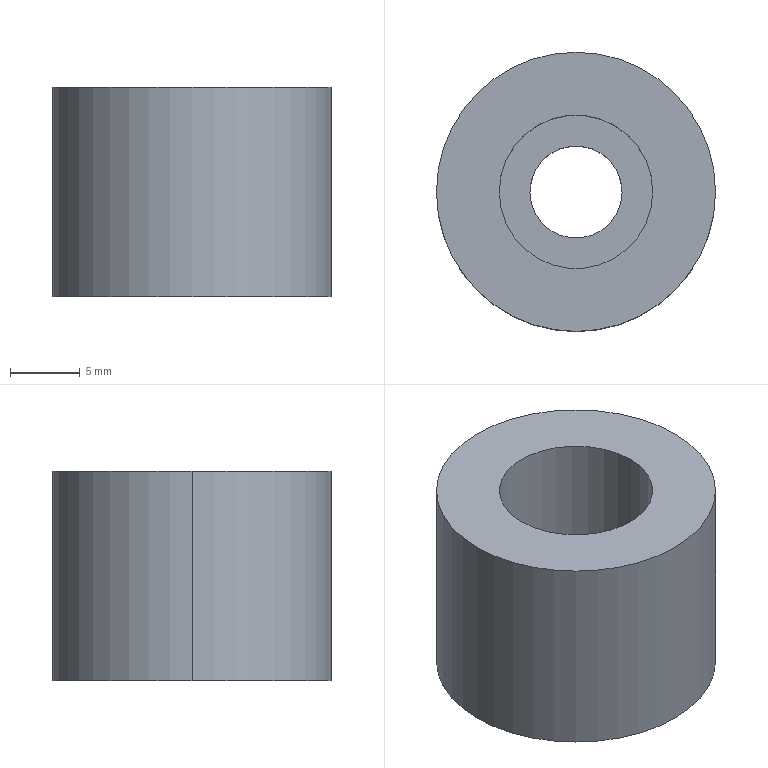Part | SolidWorks | features Extrusion 1, HoleWzd 1 | 1 solid | 9 faces | box 20 x 20 x 15 mm | volume 3713 mm3 | cylinder 6 | plane 3 | commonest cylinder face diameters 6.6 x2 11 x2 20 x2
STEP:
#1=CARTESIAN_POINT('',(-5.5,0.,7.));
#2=VERTEX_POINT('',#1);
#3=CARTESIAN_POINT('',(5.5,0.,7.));
#4=VERTEX_POINT('',#3);
#5=CARTESIAN_POINT('',(0.,0.,7.));
#6=DIRECTION('',(0.,0.,1.));
#7=DIRECTION('',(1.,0.,0.));
#8=AXIS2_PLACEMENT_3D('',#5,#6,#7);
#9=CIRCLE('',#8,5.5);
#10=EDGE_CURVE('',#2,#4,#9,.T.);
#11=ORIENTED_EDGE('',*,*,#10,.F.);
#12=CARTESIAN_POINT('',(-5.5,0.,15.));
#13=VERTEX_POINT('',#12);
#14=CARTESIAN_POINT('',(-5.5,0.,15.));
#15=DIRECTION('',(0.,0.,1.));
#16=VECTOR('',#15,1000.);
#17=LINE('',#14,#16);
#18=EDGE_CURVE('',#2,#13,#17,.T.);
#19=ORIENTED_EDGE('',*,*,#18,.T.);
#20=CARTESIAN_POINT('',(5.5,0.,15.));
#21=VERTEX_POINT('',#20);
#22=CARTESIAN_POINT('',(0.,0.,15.));
#23=DIRECTION('',(0.,0.,1.));
#24=DIRECTION('',(1.,0.,0.));
#25=AXIS2_PLACEMENT_3D('',#22,#23,#24);
#26=CIRCLE('',#25,5.5);
#27=EDGE_CURVE('',#13,#21,#26,.T.);
#28=ORIENTED_EDGE('',*,*,#27,.T.);
#29=CARTESIAN_POINT('',(5.5,0.,15.));
#30=DIRECTION('',(0.,0.,1.));
#31=VECTOR('',#30,1000.);
#32=LINE('',#29,#31);
#33=EDGE_CURVE('',#4,#21,#32,.T.);
#34=ORIENTED_EDGE('',*,*,#33,.F.);
#35=EDGE_LOOP('',(#11,#19,#28,#34));
#36=FACE_OUTER_BOUND('',#35,.T.);
#37=CARTESIAN_POINT('',(0.,0.,15.));
#38=DIRECTION('',(0.,0.,1.));
#39=DIRECTION('',(1.,0.,0.));
#40=AXIS2_PLACEMENT_3D('',#37,#38,#39);
#41=CYLINDRICAL_SURFACE('',#40,5.5);
#42=ADVANCED_FACE('',(#36),#41,.F.);
#43=CARTESIAN_POINT('',(-3.3,0.,0.));
#44=VERTEX_POINT('',#43);
#45=CARTESIAN_POINT('',(3.3,0.,0.));
#46=VERTEX_POINT('',#45);
#47=CARTESIAN_POINT('',(0.,0.,0.));
#48=DIRECTION('',(0.,0.,1.));
#49=DIRECTION('',(1.,0.,0.));
#50=AXIS2_PLACEMENT_3D('',#47,#48,#49);
#51=CIRCLE('',#50,3.3);
#52=EDGE_CURVE('',#44,#46,#51,.T.);
#53=ORIENTED_EDGE('',*,*,#52,.F.);
#54=CARTESIAN_POINT('',(-3.3,0.,7.));
#55=VERTEX_POINT('',#54);
#56=CARTESIAN_POINT('',(-3.3,0.,15.));
#57=DIRECTION('',(0.,0.,1.));
#58=VECTOR('',#57,1000.);
#59=LINE('',#56,#58);
#60=EDGE_CURVE('',#44,#55,#59,.T.);
#61=ORIENTED_EDGE('',*,*,#60,.T.);
#62=CARTESIAN_POINT('',(3.3,0.,7.));
#63=VERTEX_POINT('',#62);
#64=CARTESIAN_POINT('',(0.,0.,7.));
#65=DIRECTION('',(0.,0.,1.));
#66=DIRECTION('',(1.,0.,0.));
#67=AXIS2_PLACEMENT_3D('',#64,#65,#66);
#68=CIRCLE('',#67,3.3);
#69=EDGE_CURVE('',#55,#63,#68,.T.);
#70=ORIENTED_EDGE('',*,*,#69,.T.);
#71=CARTESIAN_POINT('',(3.3,0.,15.));
#72=DIRECTION('',(0.,0.,1.));
#73=VECTOR('',#72,1000.);
#74=LINE('',#71,#73);
#75=EDGE_CURVE('',#46,#63,#74,.T.);
#76=ORIENTED_EDGE('',*,*,#75,.F.);
#77=EDGE_LOOP('',(#53,#61,#70,#76));
#78=FACE_OUTER_BOUND('',#77,.T.);
#79=CARTESIAN_POINT('',(0.,0.,15.));
#80=DIRECTION('',(0.,0.,1.));
#81=DIRECTION('',(1.,0.,0.));
#82=AXIS2_PLACEMENT_3D('',#79,#80,#81);
#83=CYLINDRICAL_SURFACE('',#82,3.3);
#84=ADVANCED_FACE('',(#78),#83,.F.);
#85=CARTESIAN_POINT('',(10.,0.,15.));
#86=VERTEX_POINT('',#85);
#87=CARTESIAN_POINT('',(-10.,0.,15.));
#88=VERTEX_POINT('',#87);
#89=CARTESIAN_POINT('',(0.,0.,15.));
#90=DIRECTION('',(0.,0.,1.));
#91=DIRECTION('',(1.,0.,0.));
#92=AXIS2_PLACEMENT_3D('',#89,#90,#91);
#93=CIRCLE('',#92,10.);
#94=EDGE_CURVE('',#86,#88,#93,.T.);
#95=ORIENTED_EDGE('',*,*,#94,.F.);
#96=CARTESIAN_POINT('',(10.,0.,0.));
#97=VERTEX_POINT('',#96);
#98=CARTESIAN_POINT('',(10.,0.,15.));
#99=DIRECTION('',(0.,0.,-1.));
#100=VECTOR('',#99,1000.);
#101=LINE('',#98,#100);
#102=EDGE_CURVE('',#86,#97,#101,.T.);
#103=ORIENTED_EDGE('',*,*,#102,.T.);
#104=CARTESIAN_POINT('',(-10.,0.,0.));
#105=VERTEX_POINT('',#104);
#106=CARTESIAN_POINT('',(0.,0.,0.));
#107=DIRECTION('',(0.,0.,1.));
#108=DIRECTION('',(1.,0.,0.));
#109=AXIS2_PLACEMENT_3D('',#106,#107,#108);
#110=CIRCLE('',#109,10.);
#111=EDGE_CURVE('',#97,#105,#110,.T.);
#112=ORIENTED_EDGE('',*,*,#111,.T.);
#113=CARTESIAN_POINT('',(-10.,0.,15.));
#114=DIRECTION('',(0.,0.,-1.));
#115=VECTOR('',#114,1000.);
#116=LINE('',#113,#115);
#117=EDGE_CURVE('',#88,#105,#116,.T.);
#118=ORIENTED_EDGE('',*,*,#117,.F.);
#119=EDGE_LOOP('',(#95,#103,#112,#118));
#120=FACE_OUTER_BOUND('',#119,.T.);
#121=CARTESIAN_POINT('',(0.,0.,15.));
#122=DIRECTION('',(0.,0.,-1.));
#123=DIRECTION('',(-1.,0.,0.));
#124=AXIS2_PLACEMENT_3D('',#121,#122,#123);
#125=CYLINDRICAL_SURFACE('',#124,10.);
#126=ADVANCED_FACE('',(#120),#125,.T.);
#127=ORIENTED_EDGE('',*,*,#102,.F.);
#128=CARTESIAN_POINT('',(0.,0.,15.));
#129=DIRECTION('',(0.,0.,1.));
#130=DIRECTION('',(1.,0.,0.));
#131=AXIS2_PLACEMENT_3D('',#128,#129,#130);
#132=CIRCLE('',#131,10.);
#133=EDGE_CURVE('',#88,#86,#132,.T.);
#134=ORIENTED_EDGE('',*,*,#133,.F.);
#135=ORIENTED_EDGE('',*,*,#117,.T.);
#136=CARTESIAN_POINT('',(0.,0.,0.));
#137=DIRECTION('',(0.,0.,1.));
#138=DIRECTION('',(1.,0.,0.));
#139=AXIS2_PLACEMENT_3D('',#136,#137,#138);
#140=CIRCLE('',#139,10.);
#141=EDGE_CURVE('',#105,#97,#140,.T.);
#142=ORIENTED_EDGE('',*,*,#141,.T.);
#143=EDGE_LOOP('',(#127,#134,#135,#142));
#144=FACE_OUTER_BOUND('',#143,.T.);
#145=CARTESIAN_POINT('',(0.,0.,15.));
#146=DIRECTION('',(0.,0.,-1.));
#147=DIRECTION('',(-1.,0.,0.));
#148=AXIS2_PLACEMENT_3D('',#145,#146,#147);
#149=CYLINDRICAL_SURFACE('',#148,10.);
#150=ADVANCED_FACE('',(#144),#149,.T.);
#151=CARTESIAN_POINT('',(0.,0.,15.));
#152=DIRECTION('',(0.,0.,1.));
#153=DIRECTION('',(1.,0.,0.));
#154=AXIS2_PLACEMENT_3D('',#151,#152,#153);
#155=CIRCLE('',#154,5.5);
#156=EDGE_CURVE('',#21,#13,#155,.T.);
#157=ORIENTED_EDGE('',*,*,#156,.F.);
#158=ORIENTED_EDGE('',*,*,#27,.F.);
#159=EDGE_LOOP('',(#157,#158));
#160=FACE_BOUND('',#159,.T.);
#161=ORIENTED_EDGE('',*,*,#133,.T.);
#162=ORIENTED_EDGE('',*,*,#94,.T.);
#163=EDGE_LOOP('',(#161,#162));
#164=FACE_OUTER_BOUND('',#163,.T.);
#165=CARTESIAN_POINT('',(0.,0.,15.));
#166=DIRECTION('',(0.,0.,1.));
#167=DIRECTION('',(1.,0.,0.));
#168=AXIS2_PLACEMENT_3D('',#165,#166,#167);
#169=PLANE('',#168);
#170=ADVANCED_FACE('',(#160,#164),#169,.T.);
#171=CARTESIAN_POINT('',(0.,0.,0.));
#172=DIRECTION('',(0.,0.,1.));
#173=DIRECTION('',(1.,0.,0.));
#174=AXIS2_PLACEMENT_3D('',#171,#172,#173);
#175=CIRCLE('',#174,3.3);
#176=EDGE_CURVE('',#46,#44,#175,.T.);
#177=ORIENTED_EDGE('',*,*,#176,.T.);
#178=ORIENTED_EDGE('',*,*,#52,.T.);
#179=EDGE_LOOP('',(#177,#178));
#180=FACE_BOUND('',#179,.T.);
#181=ORIENTED_EDGE('',*,*,#141,.F.);
#182=ORIENTED_EDGE('',*,*,#111,.F.);
#183=EDGE_LOOP('',(#181,#182));
#184=FACE_OUTER_BOUND('',#183,.T.);
#185=CARTESIAN_POINT('',(0.,0.,0.));
#186=DIRECTION('',(0.,0.,1.));
#187=DIRECTION('',(1.,0.,0.));
#188=AXIS2_PLACEMENT_3D('',#185,#186,#187);
#189=PLANE('',#188);
#190=ADVANCED_FACE('',(#180,#184),#189,.F.);
#191=ORIENTED_EDGE('',*,*,#60,.F.);
#192=ORIENTED_EDGE('',*,*,#176,.F.);
#193=ORIENTED_EDGE('',*,*,#75,.T.);
#194=CARTESIAN_POINT('',(0.,0.,7.));
#195=DIRECTION('',(0.,0.,1.));
#196=DIRECTION('',(1.,0.,0.));
#197=AXIS2_PLACEMENT_3D('',#194,#195,#196);
#198=CIRCLE('',#197,3.3);
#199=EDGE_CURVE('',#63,#55,#198,.T.);
#200=ORIENTED_EDGE('',*,*,#199,.T.);
#201=EDGE_LOOP('',(#191,#192,#193,#200));
#202=FACE_OUTER_BOUND('',#201,.T.);
#203=CARTESIAN_POINT('',(0.,0.,15.));
#204=DIRECTION('',(0.,0.,1.));
#205=DIRECTION('',(1.,0.,0.));
#206=AXIS2_PLACEMENT_3D('',#203,#204,#205);
#207=CYLINDRICAL_SURFACE('',#206,3.3);
#208=ADVANCED_FACE('',(#202),#207,.F.);
#209=ORIENTED_EDGE('',*,*,#199,.F.);
#210=ORIENTED_EDGE('',*,*,#69,.F.);
#211=EDGE_LOOP('',(#209,#210));
#212=FACE_BOUND('',#211,.T.);
#213=CARTESIAN_POINT('',(0.,0.,7.));
#214=DIRECTION('',(0.,0.,1.));
#215=DIRECTION('',(1.,0.,0.));
#216=AXIS2_PLACEMENT_3D('',#213,#214,#215);
#217=CIRCLE('',#216,5.5);
#218=EDGE_CURVE('',#4,#2,#217,.T.);
#219=ORIENTED_EDGE('',*,*,#218,.T.);
#220=ORIENTED_EDGE('',*,*,#10,.T.);
#221=EDGE_LOOP('',(#219,#220));
#222=FACE_OUTER_BOUND('',#221,.T.);
#223=CARTESIAN_POINT('',(3.3,0.,7.));
#224=DIRECTION('',(0.,0.,-1.));
#225=DIRECTION('',(-1.,0.,0.));
#226=AXIS2_PLACEMENT_3D('',#223,#224,#225);
#227=PLANE('',#226);
#228=ADVANCED_FACE('',(#212,#222),#227,.F.);
#229=ORIENTED_EDGE('',*,*,#18,.F.);
#230=ORIENTED_EDGE('',*,*,#218,.F.);
#231=ORIENTED_EDGE('',*,*,#33,.T.);
#232=ORIENTED_EDGE('',*,*,#156,.T.);
#233=EDGE_LOOP('',(#229,#230,#231,#232));
#234=FACE_OUTER_BOUND('',#233,.T.);
#235=CARTESIAN_POINT('',(0.,0.,15.));
#236=DIRECTION('',(0.,0.,1.));
#237=DIRECTION('',(1.,0.,0.));
#238=AXIS2_PLACEMENT_3D('',#235,#236,#237);
#239=CYLINDRICAL_SURFACE('',#238,5.5);
#240=ADVANCED_FACE('',(#234),#239,.F.);
#241=CLOSED_SHELL('',(#42,#84,#126,#150,#170,#190,#208,#228,#240));
#242=MANIFOLD_SOLID_BREP('',#241);
#243=CARTESIAN_POINT('',(0.,0.,0.));
#244=DIRECTION('',(0.,0.,1.));
#245=DIRECTION('',(1.,0.,0.));
#246=AXIS2_PLACEMENT_3D('',#243,#244,#245);
#247=(LENGTH_UNIT()NAMED_UNIT(*)SI_UNIT(.MILLI.,.METRE.));
#248=UNCERTAINTY_MEASURE_WITH_UNIT(LENGTH_MEASURE(0.00001),#247,'','');
#249=(NAMED_UNIT(*)PLANE_ANGLE_UNIT()SI_UNIT($,.RADIAN.));
#250=(NAMED_UNIT(*)SI_UNIT($,.STERADIAN.)SOLID_ANGLE_UNIT());
#251=(GEOMETRIC_REPRESENTATION_CONTEXT(3)GLOBAL_UNCERTAINTY_ASSIGNED_CONTEXT((#248))GLOBAL_UNIT_ASSIGNED_CONTEXT((#247,#249,#250))REPRESENTATION_CONTEXT('',''));
#252=ADVANCED_BREP_SHAPE_REPRESENTATION('',(#242,#246),#251);